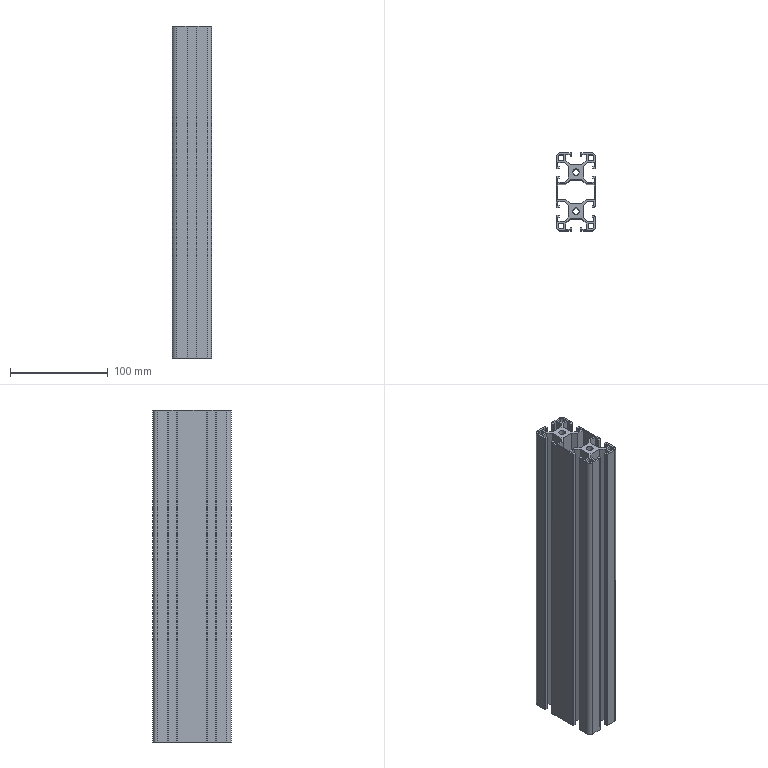Part | SolidWorks | features BaseBody 1 | 1 solid | 155 faces | box 40.002 x 80 x 340 mm | volume 334694 mm3 | plane 142 | cylinder 13 | commonest cylinder face diameters 9 x5 5 x4 6.8 x4